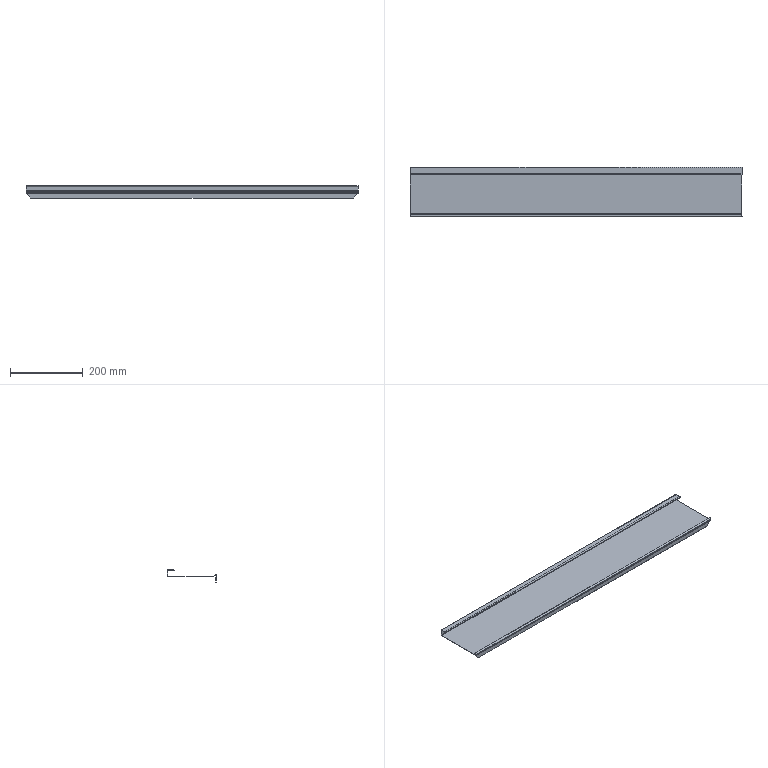Part | SolidWorks | features SM3dBend 4, EdgeFlange 2, FlatPattern 1, Hem 1, SMBaseFlange 1, SheetMetal 1 | 1 solid | 64 faces | box 915 x 136.571 x 33.2 mm | volume 145674 mm3 | plane 48 | cylinder 14 | spline 2 | commonest cylinder face diameters 1 x3 2.6 x3 0.1 x1 1.2 x1 1.7 x1 2.8 x1